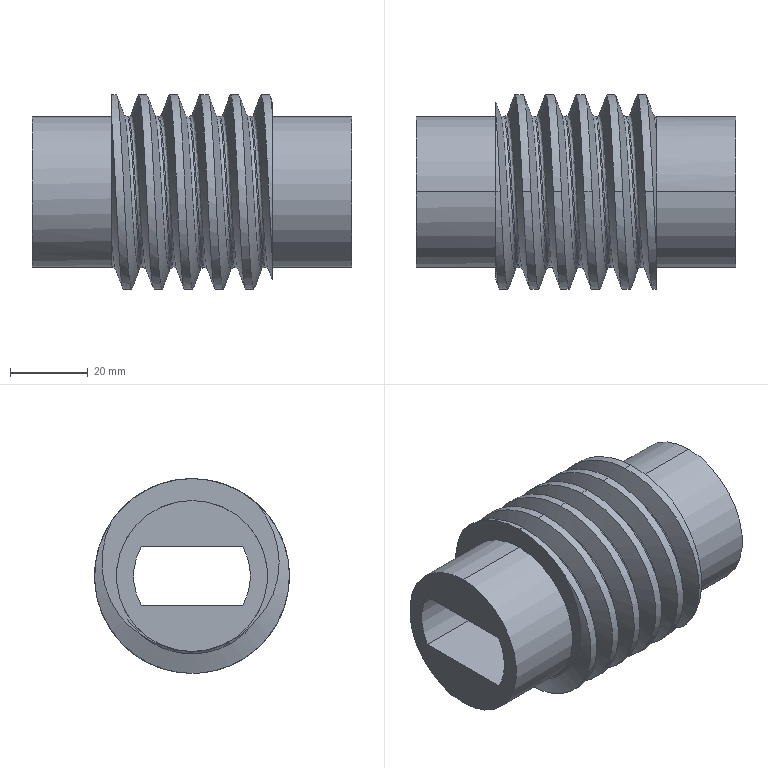Part | SolidWorks | 1 solid | 30 faces | box 82 x 50 x 50 mm | volume 78196 mm3 | cylinder 19 | plane 6 | spline 5 | commonest cylinder face diameters 50 x12 38.75 x4 30 x3